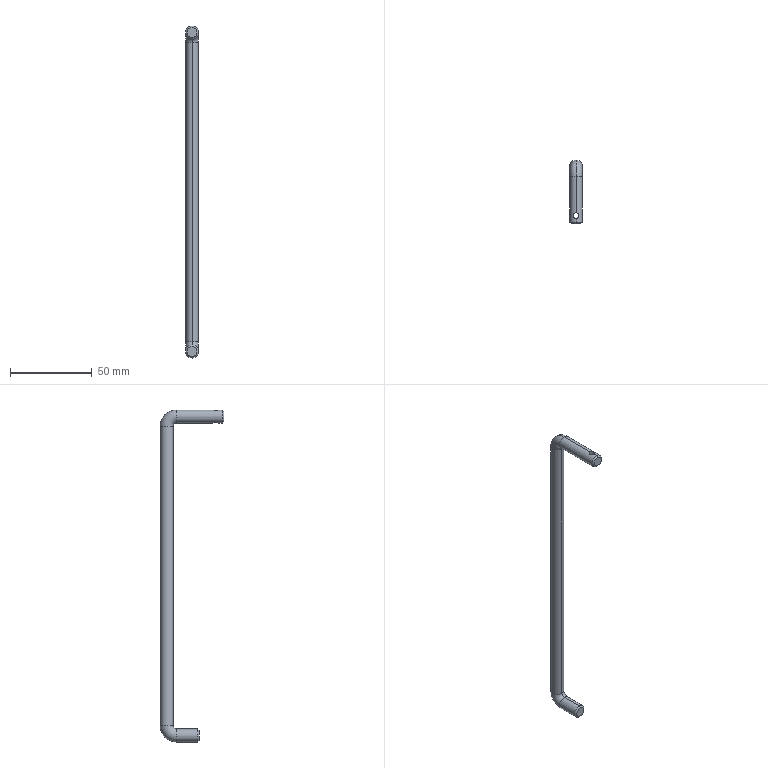Part | SolidWorks | features BaseBody 1 | 1 solid | 18 faces | box 8 x 39 x 203 mm | volume 12209 mm3 | cylinder 8 | cone 4 | torus 4 | plane 2 | commonest cylinder face diameters 8 x6 3.5 x2
STEP:
#1=CARTESIAN_POINT('',(1.75,-30.,101.097));
#2=VERTEX_POINT('',#1);
#3=CARTESIAN_POINT('',(1.75,-30.,93.903));
#4=VERTEX_POINT('',#3);
#5=CARTESIAN_POINT('',(1.75,-30.,132.));
#6=DIRECTION('',(0.,0.,-1.));
#7=VECTOR('',#6,1000.);
#8=LINE('',#5,#7);
#9=EDGE_CURVE('',#2,#4,#8,.T.);
#10=ORIENTED_EDGE('',*,*,#9,.F.);
#11=CARTESIAN_POINT('',(0.,-28.25,101.5));
#12=VERTEX_POINT('',#11);
#13=CARTESIAN_POINT('',(0.,-28.25,101.5));
#14=CARTESIAN_POINT('',(0.1167,-28.25,101.5));
#15=CARTESIAN_POINT('',(0.2317,-28.261,101.495));
#16=CARTESIAN_POINT('',(0.4573,-28.307,101.475));
#17=CARTESIAN_POINT('',(0.5697,-28.341,101.461));
#18=CARTESIAN_POINT('',(0.8889,-28.475,101.406));
#19=CARTESIAN_POINT('',(1.075,-28.6,101.357));
#20=CARTESIAN_POINT('',(1.321,-28.847,101.276));
#21=CARTESIAN_POINT('',(1.393,-28.935,101.25));
#22=CARTESIAN_POINT('',(1.487,-29.075,101.213));
#23=CARTESIAN_POINT('',(1.516,-29.124,101.202));
#24=CARTESIAN_POINT('',(1.569,-29.223,101.179));
#25=CARTESIAN_POINT('',(1.593,-29.272,101.169));
#26=CARTESIAN_POINT('',(1.706,-29.544,101.119));
#27=CARTESIAN_POINT('',(1.75,-29.768,101.097));
#28=CARTESIAN_POINT('',(1.75,-30.,101.097));
#29=B_SPLINE_CURVE_WITH_KNOTS('',3,(#13,#14,#15,#16,#17,#18,#19,#20,#21,#22,#23,#24,#25,#26,#27,#28),.UNSPECIFIED.,.F.,.F.,(4,2,2,2,2,2,2,4),(0.,0.125,0.25,0.5,0.625,0.6875,0.75,1.),.UNSPECIFIED.);
#30=EDGE_CURVE('',#12,#2,#29,.T.);
#31=ORIENTED_EDGE('',*,*,#30,.F.);
#32=CARTESIAN_POINT('',(-1.75,-30.,101.097));
#33=VERTEX_POINT('',#32);
#34=CARTESIAN_POINT('',(-1.75,-30.,101.097));
#35=CARTESIAN_POINT('',(-1.75,-29.884,101.097));
#36=CARTESIAN_POINT('',(-1.739,-29.769,101.102));
#37=CARTESIAN_POINT('',(-1.705,-29.6,101.118));
#38=CARTESIAN_POINT('',(-1.691,-29.545,101.125));
#39=CARTESIAN_POINT('',(-1.666,-29.462,101.137));
#40=CARTESIAN_POINT('',(-1.656,-29.434,101.141));
#41=CARTESIAN_POINT('',(-1.636,-29.379,101.15));
#42=CARTESIAN_POINT('',(-1.625,-29.351,101.155));
#43=CARTESIAN_POINT('',(-1.571,-29.22,101.179));
#44=CARTESIAN_POINT('',(-1.516,-29.118,101.202));
#45=CARTESIAN_POINT('',(-1.389,-28.93,101.252));
#46=CARTESIAN_POINT('',(-1.317,-28.842,101.278));
#47=CARTESIAN_POINT('',(-1.157,-28.683,101.33));
#48=CARTESIAN_POINT('',(-1.07,-28.611,101.355));
#49=CARTESIAN_POINT('',(-0.9274,-28.515,101.391));
#50=CARTESIAN_POINT('',(-0.8785,-28.486,101.403));
#51=CARTESIAN_POINT('',(-0.7783,-28.432,101.424));
#52=CARTESIAN_POINT('',(-0.7286,-28.408,101.433));
#53=CARTESIAN_POINT('',(-0.4588,-28.295,101.48));
#54=CARTESIAN_POINT('',(-0.233,-28.25,101.5));
#55=CARTESIAN_POINT('',(0.,-28.25,101.5));
#56=B_SPLINE_CURVE_WITH_KNOTS('',3,(#34,#35,#36,#37,#38,#39,#40,#41,#42,#43,#44,#45,#46,#47,#48,#49,#50,#51,#52,#53,#54,#55),.UNSPECIFIED.,.F.,.F.,(4,2,2,2,2,2,2,2,2,2,4),(0.,0.125,0.1875,0.2187,0.25,0.375,0.5,0.625,0.6875,0.75,1.),.UNSPECIFIED.);
#57=EDGE_CURVE('',#33,#12,#56,.T.);
#58=ORIENTED_EDGE('',*,*,#57,.F.);
#59=CARTESIAN_POINT('',(-1.75,-30.,93.903));
#60=VERTEX_POINT('',#59);
#61=CARTESIAN_POINT('',(-1.75,-30.,132.));
#62=DIRECTION('',(0.,0.,-1.));
#63=VECTOR('',#62,1000.);
#64=LINE('',#61,#63);
#65=EDGE_CURVE('',#33,#60,#64,.T.);
#66=ORIENTED_EDGE('',*,*,#65,.T.);
#67=CARTESIAN_POINT('',(0.,-28.25,93.5));
#68=VERTEX_POINT('',#67);
#69=CARTESIAN_POINT('',(0.,-28.25,93.5));
#70=CARTESIAN_POINT('',(-0.1167,-28.25,93.5));
#71=CARTESIAN_POINT('',(-0.2317,-28.261,93.505));
#72=CARTESIAN_POINT('',(-0.4008,-28.295,93.52));
#73=CARTESIAN_POINT('',(-0.4567,-28.309,93.526));
#74=CARTESIAN_POINT('',(-0.5672,-28.343,93.54));
#75=CARTESIAN_POINT('',(-0.6233,-28.364,93.549));
#76=CARTESIAN_POINT('',(-0.7812,-28.43,93.576));
#77=CARTESIAN_POINT('',(-0.8823,-28.485,93.597));
#78=CARTESIAN_POINT('',(-1.072,-28.612,93.645));
#79=CARTESIAN_POINT('',(-1.159,-28.684,93.671));
#80=CARTESIAN_POINT('',(-1.319,-28.844,93.723));
#81=CARTESIAN_POINT('',(-1.39,-28.93,93.748));
#82=CARTESIAN_POINT('',(-1.486,-29.074,93.786));
#83=CARTESIAN_POINT('',(-1.515,-29.123,93.798));
#84=CARTESIAN_POINT('',(-1.556,-29.198,93.815));
#85=CARTESIAN_POINT('',(-1.568,-29.223,93.82));
#86=CARTESIAN_POINT('',(-1.593,-29.274,93.831));
#87=CARTESIAN_POINT('',(-1.604,-29.299,93.836));
#88=CARTESIAN_POINT('',(-1.706,-29.543,93.881));
#89=CARTESIAN_POINT('',(-1.75,-29.768,93.903));
#90=CARTESIAN_POINT('',(-1.75,-30.,93.903));
#91=B_SPLINE_CURVE_WITH_KNOTS('',3,(#69,#70,#71,#72,#73,#74,#75,#76,#77,#78,#79,#80,#81,#82,#83,#84,#85,#86,#87,#88,#89,#90),.UNSPECIFIED.,.F.,.F.,(4,2,2,2,2,2,2,2,2,2,4),(0.,0.125,0.1875,0.25,0.375,0.5,0.625,0.6875,0.7187,0.75,1.),.UNSPECIFIED.);
#92=EDGE_CURVE('',#68,#60,#91,.T.);
#93=ORIENTED_EDGE('',*,*,#92,.F.);
#94=CARTESIAN_POINT('',(1.75,-30.,93.903));
#95=CARTESIAN_POINT('',(1.75,-29.77,93.903));
#96=CARTESIAN_POINT('',(1.703,-29.536,93.879));
#97=CARTESIAN_POINT('',(1.571,-29.221,93.821));
#98=CARTESIAN_POINT('',(1.518,-29.121,93.799));
#99=CARTESIAN_POINT('',(1.393,-28.934,93.75));
#100=CARTESIAN_POINT('',(1.319,-28.844,93.723));
#101=CARTESIAN_POINT('',(1.157,-28.682,93.67));
#102=CARTESIAN_POINT('',(1.069,-28.61,93.644));
#103=CARTESIAN_POINT('',(0.8816,-28.484,93.597));
#104=CARTESIAN_POINT('',(0.7831,-28.431,93.576));
#105=CARTESIAN_POINT('',(0.4592,-28.295,93.52));
#106=CARTESIAN_POINT('',(0.2331,-28.25,93.5));
#107=CARTESIAN_POINT('',(0.,-28.25,93.5));
#108=B_SPLINE_CURVE_WITH_KNOTS('',3,(#94,#95,#96,#97,#98,#99,#100,#101,#102,#103,#104,#105,#106,#107),.UNSPECIFIED.,.F.,.F.,(4,2,2,2,2,2,4),(0.,0.25,0.375,0.5,0.625,0.75,1.),.UNSPECIFIED.);
#109=EDGE_CURVE('',#4,#68,#108,.T.);
#110=ORIENTED_EDGE('',*,*,#109,.F.);
#111=EDGE_LOOP('',(#10,#31,#58,#66,#93,#110));
#112=FACE_OUTER_BOUND('',#111,.T.);
#113=CARTESIAN_POINT('',(0.,-30.,132.));
#114=DIRECTION('',(0.,0.,-1.));
#115=DIRECTION('',(-1.,0.,0.));
#116=AXIS2_PLACEMENT_3D('',#113,#114,#115);
#117=CYLINDRICAL_SURFACE('',#116,1.75);
#118=ADVANCED_FACE('',(#112),#117,.F.);
#119=CARTESIAN_POINT('',(0.,-35.,94.5));
#120=VERTEX_POINT('',#119);
#121=CARTESIAN_POINT('',(0.,-34.,93.5));
#122=VERTEX_POINT('',#121);
#123=CARTESIAN_POINT('',(0.,-35.,94.5));
#124=DIRECTION('',(0.,0.7071,-0.7071));
#125=VECTOR('',#124,1000.);
#126=LINE('',#123,#125);
#127=EDGE_CURVE('',#120,#122,#126,.T.);
#128=ORIENTED_EDGE('',*,*,#127,.F.);
#129=CARTESIAN_POINT('',(0.,-35.,100.5));
#130=VERTEX_POINT('',#129);
#131=CARTESIAN_POINT('',(0.,-35.,97.5));
#132=DIRECTION('',(0.,-1.,0.));
#133=DIRECTION('',(0.,0.,-1.));
#134=AXIS2_PLACEMENT_3D('',#131,#132,#133);
#135=CIRCLE('',#134,3.);
#136=EDGE_CURVE('',#130,#120,#135,.T.);
#137=ORIENTED_EDGE('',*,*,#136,.F.);
#138=CARTESIAN_POINT('',(0.,-34.,101.5));
#139=VERTEX_POINT('',#138);
#140=CARTESIAN_POINT('',(0.,-35.,100.5));
#141=DIRECTION('',(0.,0.7071,0.7071));
#142=VECTOR('',#141,1000.);
#143=LINE('',#140,#142);
#144=EDGE_CURVE('',#130,#139,#143,.T.);
#145=ORIENTED_EDGE('',*,*,#144,.T.);
#146=CARTESIAN_POINT('',(0.,-34.,97.5));
#147=DIRECTION('',(0.,1.,0.));
#148=DIRECTION('',(0.,0.,-1.));
#149=AXIS2_PLACEMENT_3D('',#146,#147,#148);
#150=CIRCLE('',#149,4.);
#151=EDGE_CURVE('',#122,#139,#150,.T.);
#152=ORIENTED_EDGE('',*,*,#151,.F.);
#153=EDGE_LOOP('',(#128,#137,#145,#152));
#154=FACE_OUTER_BOUND('',#153,.T.);
#155=CARTESIAN_POINT('',(0.,-35.,97.5));
#156=DIRECTION('',(0.,1.,0.));
#157=DIRECTION('',(0.,0.,1.));
#158=AXIS2_PLACEMENT_3D('',#155,#156,#157);
#159=CONICAL_SURFACE('',#158,3.,0.7854);
#160=ADVANCED_FACE('',(#154),#159,.T.);
#161=CARTESIAN_POINT('',(0.,-20.,-100.5));
#162=VERTEX_POINT('',#161);
#163=CARTESIAN_POINT('',(0.,-19.,-101.5));
#164=VERTEX_POINT('',#163);
#165=CARTESIAN_POINT('',(0.,-19.,-101.5));
#166=DIRECTION('',(0.,0.7071,-0.7071));
#167=VECTOR('',#166,1000.);
#168=LINE('',#165,#167);
#169=EDGE_CURVE('',#162,#164,#168,.T.);
#170=ORIENTED_EDGE('',*,*,#169,.F.);
#171=CARTESIAN_POINT('',(0.,-20.,-94.5));
#172=VERTEX_POINT('',#171);
#173=CARTESIAN_POINT('',(0.,-20.,-97.5));
#174=DIRECTION('',(0.,-1.,0.));
#175=DIRECTION('',(0.,0.,1.));
#176=AXIS2_PLACEMENT_3D('',#173,#174,#175);
#177=CIRCLE('',#176,3.);
#178=EDGE_CURVE('',#172,#162,#177,.T.);
#179=ORIENTED_EDGE('',*,*,#178,.F.);
#180=CARTESIAN_POINT('',(0.,-19.,-93.5));
#181=VERTEX_POINT('',#180);
#182=CARTESIAN_POINT('',(0.,-19.,-93.5));
#183=DIRECTION('',(0.,0.7071,0.7071));
#184=VECTOR('',#183,1000.);
#185=LINE('',#182,#184);
#186=EDGE_CURVE('',#172,#181,#185,.T.);
#187=ORIENTED_EDGE('',*,*,#186,.T.);
#188=CARTESIAN_POINT('',(0.,-19.,-97.5));
#189=DIRECTION('',(0.,1.,0.));
#190=DIRECTION('',(0.,0.,1.));
#191=AXIS2_PLACEMENT_3D('',#188,#189,#190);
#192=CIRCLE('',#191,4.);
#193=EDGE_CURVE('',#164,#181,#192,.T.);
#194=ORIENTED_EDGE('',*,*,#193,.F.);
#195=EDGE_LOOP('',(#170,#179,#187,#194));
#196=FACE_OUTER_BOUND('',#195,.T.);
#197=CARTESIAN_POINT('',(0.,-19.,-97.5));
#198=DIRECTION('',(0.,1.,0.));
#199=DIRECTION('',(0.,0.,1.));
#200=AXIS2_PLACEMENT_3D('',#197,#198,#199);
#201=CONICAL_SURFACE('',#200,4.,0.7854);
#202=ADVANCED_FACE('',(#196),#201,.T.);
#203=ORIENTED_EDGE('',*,*,#178,.T.);
#204=CARTESIAN_POINT('',(0.,-20.,-97.5));
#205=DIRECTION('',(0.,-1.,0.));
#206=DIRECTION('',(0.,0.,1.));
#207=AXIS2_PLACEMENT_3D('',#204,#205,#206);
#208=CIRCLE('',#207,3.);
#209=EDGE_CURVE('',#162,#172,#208,.T.);
#210=ORIENTED_EDGE('',*,*,#209,.T.);
#211=EDGE_LOOP('',(#203,#210));
#212=FACE_OUTER_BOUND('',#211,.T.);
#213=CARTESIAN_POINT('',(0.,-20.,-97.5));
#214=DIRECTION('',(0.,1.,0.));
#215=DIRECTION('',(0.,0.,-1.));
#216=AXIS2_PLACEMENT_3D('',#213,#214,#215);
#217=PLANE('',#216);
#218=ADVANCED_FACE('',(#212),#217,.F.);
#219=ORIENTED_EDGE('',*,*,#136,.T.);
#220=CARTESIAN_POINT('',(0.,-35.,97.5));
#221=DIRECTION('',(0.,-1.,0.));
#222=DIRECTION('',(0.,0.,-1.));
#223=AXIS2_PLACEMENT_3D('',#220,#221,#222);
#224=CIRCLE('',#223,3.);
#225=EDGE_CURVE('',#120,#130,#224,.T.);
#226=ORIENTED_EDGE('',*,*,#225,.T.);
#227=EDGE_LOOP('',(#219,#226));
#228=FACE_OUTER_BOUND('',#227,.T.);
#229=CARTESIAN_POINT('',(0.,-35.,97.5));
#230=DIRECTION('',(0.,-1.,0.));
#231=DIRECTION('',(0.,0.,-1.));
#232=AXIS2_PLACEMENT_3D('',#229,#230,#231);
#233=PLANE('',#232);
#234=ADVANCED_FACE('',(#228),#233,.T.);
#235=CARTESIAN_POINT('',(0.,-6.,-101.5));
#236=VERTEX_POINT('',#235);
#237=CARTESIAN_POINT('',(0.,-20.,-101.5));
#238=DIRECTION('',(0.,1.,0.));
#239=VECTOR('',#238,1000.);
#240=LINE('',#237,#239);
#241=EDGE_CURVE('',#164,#236,#240,.T.);
#242=ORIENTED_EDGE('',*,*,#241,.F.);
#243=ORIENTED_EDGE('',*,*,#193,.T.);
#244=CARTESIAN_POINT('',(0.,-6.,-93.5));
#245=VERTEX_POINT('',#244);
#246=CARTESIAN_POINT('',(0.,-20.,-93.5));
#247=DIRECTION('',(0.,1.,0.));
#248=VECTOR('',#247,1000.);
#249=LINE('',#246,#248);
#250=EDGE_CURVE('',#181,#245,#249,.T.);
#251=ORIENTED_EDGE('',*,*,#250,.T.);
#252=CARTESIAN_POINT('',(0.,-6.,-97.5));
#253=DIRECTION('',(0.,1.,0.));
#254=DIRECTION('',(1.,0.,0.));
#255=AXIS2_PLACEMENT_3D('',#252,#253,#254);
#256=CIRCLE('',#255,4.);
#257=EDGE_CURVE('',#236,#245,#256,.T.);
#258=ORIENTED_EDGE('',*,*,#257,.F.);
#259=EDGE_LOOP('',(#242,#243,#251,#258));
#260=FACE_OUTER_BOUND('',#259,.T.);
#261=CARTESIAN_POINT('',(0.,-20.,-97.5));
#262=DIRECTION('',(0.,1.,0.));
#263=DIRECTION('',(0.,0.,1.));
#264=AXIS2_PLACEMENT_3D('',#261,#262,#263);
#265=CYLINDRICAL_SURFACE('',#264,4.);
#266=ADVANCED_FACE('',(#260),#265,.T.);
#267=CARTESIAN_POINT('',(0.,4.,-91.5));
#268=VERTEX_POINT('',#267);
#269=CARTESIAN_POINT('',(0.,-6.,-91.5));
#270=DIRECTION('',(1.,0.,0.));
#271=DIRECTION('',(0.,0.,-1.));
#272=AXIS2_PLACEMENT_3D('',#269,#270,#271);
#273=CIRCLE('',#272,10.);
#274=EDGE_CURVE('',#236,#268,#273,.T.);
#275=ORIENTED_EDGE('',*,*,#274,.F.);
#276=ORIENTED_EDGE('',*,*,#257,.T.);
#277=CARTESIAN_POINT('',(0.,-4.,-91.5));
#278=VERTEX_POINT('',#277);
#279=CARTESIAN_POINT('',(0.,-6.,-91.5));
#280=DIRECTION('',(1.,0.,0.));
#281=DIRECTION('',(0.,0.,-1.));
#282=AXIS2_PLACEMENT_3D('',#279,#280,#281);
#283=CIRCLE('',#282,2.);
#284=EDGE_CURVE('',#245,#278,#283,.T.);
#285=ORIENTED_EDGE('',*,*,#284,.T.);
#286=CARTESIAN_POINT('',(0.,0.,-91.5));
#287=DIRECTION('',(0.,0.,1.));
#288=DIRECTION('',(1.,0.,0.));
#289=AXIS2_PLACEMENT_3D('',#286,#287,#288);
#290=CIRCLE('',#289,4.);
#291=EDGE_CURVE('',#268,#278,#290,.T.);
#292=ORIENTED_EDGE('',*,*,#291,.F.);
#293=EDGE_LOOP('',(#275,#276,#285,#292));
#294=FACE_OUTER_BOUND('',#293,.T.);
#295=CARTESIAN_POINT('',(0.,-6.,-91.5));
#296=DIRECTION('',(1.,0.,0.));
#297=DIRECTION('',(0.,0.,-1.));
#298=AXIS2_PLACEMENT_3D('',#295,#296,#297);
#299=TOROIDAL_SURFACE('',#298,6.,4.);
#300=ADVANCED_FACE('',(#294),#299,.T.);
#301=CARTESIAN_POINT('',(0.,4.,91.5));
#302=VERTEX_POINT('',#301);
#303=CARTESIAN_POINT('',(0.,4.,-91.5));
#304=DIRECTION('',(0.,0.,1.));
#305=VECTOR('',#304,1000.);
#306=LINE('',#303,#305);
#307=EDGE_CURVE('',#268,#302,#306,.T.);
#308=ORIENTED_EDGE('',*,*,#307,.F.);
#309=ORIENTED_EDGE('',*,*,#291,.T.);
#310=CARTESIAN_POINT('',(0.,-4.,91.5));
#311=VERTEX_POINT('',#310);
#312=CARTESIAN_POINT('',(0.,-4.,-91.5));
#313=DIRECTION('',(0.,0.,1.));
#314=VECTOR('',#313,1000.);
#315=LINE('',#312,#314);
#316=EDGE_CURVE('',#278,#311,#315,.T.);
#317=ORIENTED_EDGE('',*,*,#316,.T.);
#318=CARTESIAN_POINT('',(0.,0.,91.5));
#319=DIRECTION('',(0.,0.,1.));
#320=DIRECTION('',(1.,0.,0.));
#321=AXIS2_PLACEMENT_3D('',#318,#319,#320);
#322=CIRCLE('',#321,4.);
#323=EDGE_CURVE('',#302,#311,#322,.T.);
#324=ORIENTED_EDGE('',*,*,#323,.F.);
#325=EDGE_LOOP('',(#308,#309,#317,#324));
#326=FACE_OUTER_BOUND('',#325,.T.);
#327=CARTESIAN_POINT('',(0.,0.,-91.5));
#328=DIRECTION('',(0.,0.,1.));
#329=DIRECTION('',(0.,-1.,0.));
#330=AXIS2_PLACEMENT_3D('',#327,#328,#329);
#331=CYLINDRICAL_SURFACE('',#330,4.);
#332=ADVANCED_FACE('',(#326),#331,.T.);
#333=CARTESIAN_POINT('',(0.,-6.,101.5));
#334=VERTEX_POINT('',#333);
#335=CARTESIAN_POINT('',(0.,-6.,91.5));
#336=DIRECTION('',(1.,0.,0.));
#337=DIRECTION('',(0.,0.,-1.));
#338=AXIS2_PLACEMENT_3D('',#335,#336,#337);
#339=CIRCLE('',#338,10.);
#340=EDGE_CURVE('',#302,#334,#339,.T.);
#341=ORIENTED_EDGE('',*,*,#340,.F.);
#342=ORIENTED_EDGE('',*,*,#323,.T.);
#343=CARTESIAN_POINT('',(0.,-6.,93.5));
#344=VERTEX_POINT('',#343);
#345=CARTESIAN_POINT('',(0.,-6.,91.5));
#346=DIRECTION('',(1.,0.,0.));
#347=DIRECTION('',(0.,0.,-1.));
#348=AXIS2_PLACEMENT_3D('',#345,#346,#347);
#349=CIRCLE('',#348,2.);
#350=EDGE_CURVE('',#311,#344,#349,.T.);
#351=ORIENTED_EDGE('',*,*,#350,.T.);
#352=CARTESIAN_POINT('',(0.,-6.,97.5));
#353=DIRECTION('',(0.,-1.,0.));
#354=DIRECTION('',(1.,0.,0.));
#355=AXIS2_PLACEMENT_3D('',#352,#353,#354);
#356=CIRCLE('',#355,4.);
#357=EDGE_CURVE('',#334,#344,#356,.T.);
#358=ORIENTED_EDGE('',*,*,#357,.F.);
#359=EDGE_LOOP('',(#341,#342,#351,#358));
#360=FACE_OUTER_BOUND('',#359,.T.);
#361=CARTESIAN_POINT('',(0.,-6.,91.5));
#362=DIRECTION('',(1.,0.,0.));
#363=DIRECTION('',(0.,0.,-1.));
#364=AXIS2_PLACEMENT_3D('',#361,#362,#363);
#365=TOROIDAL_SURFACE('',#364,6.,4.);
#366=ADVANCED_FACE('',(#360),#365,.T.);
#367=CARTESIAN_POINT('',(0.,-6.,101.5));
#368=DIRECTION('',(0.,-1.,0.));
#369=VECTOR('',#368,1000.);
#370=LINE('',#367,#369);
#371=EDGE_CURVE('',#334,#12,#370,.T.);
#372=ORIENTED_EDGE('',*,*,#371,.F.);
#373=ORIENTED_EDGE('',*,*,#357,.T.);
#374=CARTESIAN_POINT('',(0.,-6.,93.5));
#375=DIRECTION('',(0.,-1.,0.));
#376=VECTOR('',#375,1000.);
#377=LINE('',#374,#376);
#378=EDGE_CURVE('',#344,#68,#377,.T.);
#379=ORIENTED_EDGE('',*,*,#378,.T.);
#380=ORIENTED_EDGE('',*,*,#92,.T.);
#381=CARTESIAN_POINT('',(0.,-31.75,93.5));
#382=VERTEX_POINT('',#381);
#383=CARTESIAN_POINT('',(-1.75,-30.,93.903));
#384=CARTESIAN_POINT('',(-1.75,-30.116,93.903));
#385=CARTESIAN_POINT('',(-1.739,-30.231,93.898));
#386=CARTESIAN_POINT('',(-1.705,-30.4,93.882));
#387=CARTESIAN_POINT('',(-1.691,-30.455,93.875));
#388=CARTESIAN_POINT('',(-1.657,-30.566,93.859));
#389=CARTESIAN_POINT('',(-1.636,-30.623,93.85));
#390=CARTESIAN_POINT('',(-1.57,-30.781,93.821));
#391=CARTESIAN_POINT('',(-1.517,-30.88,93.798));
#392=CARTESIAN_POINT('',(-1.392,-31.068,93.749));
#393=CARTESIAN_POINT('',(-1.318,-31.157,93.722));
#394=CARTESIAN_POINT('',(-1.155,-31.319,93.67));
#395=CARTESIAN_POINT('',(-1.068,-31.391,93.644));
#396=CARTESIAN_POINT('',(-0.8804,-31.517,93.597));
#397=CARTESIAN_POINT('',(-0.7819,-31.57,93.576));
#398=CARTESIAN_POINT('',(-0.4584,-31.705,93.52));
#399=CARTESIAN_POINT('',(-0.2328,-31.75,93.5));
#400=CARTESIAN_POINT('',(0.,-31.75,93.5));
#401=B_SPLINE_CURVE_WITH_KNOTS('',3,(#383,#384,#385,#386,#387,#388,#389,#390,#391,#392,#393,#394,#395,#396,#397,#398,#399,#400),.UNSPECIFIED.,.F.,.F.,(4,2,2,2,2,2,2,2,4),(0.,0.125,0.1875,0.25,0.375,0.5,0.625,0.75,1.),.UNSPECIFIED.);
#402=EDGE_CURVE('',#60,#382,#401,.T.);
#403=ORIENTED_EDGE('',*,*,#402,.T.);
#404=CARTESIAN_POINT('',(0.,-6.,93.5));
#405=DIRECTION('',(0.,-1.,0.));
#406=VECTOR('',#405,1000.);
#407=LINE('',#404,#406);
#408=EDGE_CURVE('',#382,#122,#407,.T.);
#409=ORIENTED_EDGE('',*,*,#408,.T.);
#410=ORIENTED_EDGE('',*,*,#151,.T.);
#411=CARTESIAN_POINT('',(0.,-31.75,101.5));
#412=VERTEX_POINT('',#411);
#413=CARTESIAN_POINT('',(0.,-6.,101.5));
#414=DIRECTION('',(0.,-1.,0.));
#415=VECTOR('',#414,1000.);
#416=LINE('',#413,#415);
#417=EDGE_CURVE('',#412,#139,#416,.T.);
#418=ORIENTED_EDGE('',*,*,#417,.F.);
#419=CARTESIAN_POINT('',(0.,-31.75,101.5));
#420=CARTESIAN_POINT('',(-0.1165,-31.75,101.5));
#421=CARTESIAN_POINT('',(-0.2312,-31.739,101.495));
#422=CARTESIAN_POINT('',(-0.4563,-31.694,101.475));
#423=CARTESIAN_POINT('',(-0.5683,-31.659,101.461));
#424=CARTESIAN_POINT('',(-0.7811,-31.57,101.424));
#425=CARTESIAN_POINT('',(-0.8813,-31.517,101.403));
#426=CARTESIAN_POINT('',(-1.069,-31.391,101.356));
#427=CARTESIAN_POINT('',(-1.156,-31.319,101.33));
#428=CARTESIAN_POINT('',(-1.32,-31.155,101.277));
#429=CARTESIAN_POINT('',(-1.393,-31.066,101.25));
#430=CARTESIAN_POINT('',(-1.486,-30.926,101.214));
#431=CARTESIAN_POINT('',(-1.515,-30.878,101.202));
#432=CARTESIAN_POINT('',(-1.569,-30.778,101.18));
#433=CARTESIAN_POINT('',(-1.592,-30.729,101.17));
#434=CARTESIAN_POINT('',(-1.706,-30.457,101.119));
#435=CARTESIAN_POINT('',(-1.75,-30.232,101.097));
#436=CARTESIAN_POINT('',(-1.75,-30.,101.097));
#437=B_SPLINE_CURVE_WITH_KNOTS('',3,(#419,#420,#421,#422,#423,#424,#425,#426,#427,#428,#429,#430,#431,#432,#433,#434,#435,#436),.UNSPECIFIED.,.F.,.F.,(4,2,2,2,2,2,2,2,4),(0.,0.125,0.25,0.375,0.5,0.625,0.6875,0.75,1.),.UNSPECIFIED.);
#438=EDGE_CURVE('',#412,#33,#437,.T.);
#439=ORIENTED_EDGE('',*,*,#438,.T.);
#440=ORIENTED_EDGE('',*,*,#57,.T.);
#441=EDGE_LOOP('',(#372,#373,#379,#380,#403,#409,#410,#418,#439,#440));
#442=FACE_OUTER_BOUND('',#441,.T.);
#443=CARTESIAN_POINT('',(0.,-6.,97.5));
#444=DIRECTION('',(0.,-1.,0.));
#445=DIRECTION('',(0.,0.,-1.));
#446=AXIS2_PLACEMENT_3D('',#443,#444,#445);
#447=CYLINDRICAL_SURFACE('',#446,4.);
#448=ADVANCED_FACE('',(#442),#447,.T.);
#449=CARTESIAN_POINT('',(0.,-6.,97.5));
#450=DIRECTION('',(0.,-1.,0.));
#451=DIRECTION('',(1.,0.,0.));
#452=AXIS2_PLACEMENT_3D('',#449,#450,#451);
#453=CIRCLE('',#452,4.);
#454=EDGE_CURVE('',#344,#334,#453,.T.);
#455=ORIENTED_EDGE('',*,*,#454,.T.);
#456=ORIENTED_EDGE('',*,*,#371,.T.);
#457=ORIENTED_EDGE('',*,*,#30,.T.);
#458=CARTESIAN_POINT('',(1.75,-30.,101.097));
#459=CARTESIAN_POINT('',(1.75,-30.116,101.097));
#460=CARTESIAN_POINT('',(1.739,-30.23,101.102));
#461=CARTESIAN_POINT('',(1.705,-30.399,101.118));
#462=CARTESIAN_POINT('',(1.691,-30.455,101.125));
#463=CARTESIAN_POINT('',(1.657,-30.565,101.141));
#464=CARTESIAN_POINT('',(1.637,-30.622,101.15));
#465=CARTESIAN_POINT('',(1.571,-30.78,101.179));
#466=CARTESIAN_POINT('',(1.518,-30.88,101.202));
#467=CARTESIAN_POINT('',(1.392,-31.067,101.251));
#468=CARTESIAN_POINT('',(1.318,-31.157,101.277));
#469=CARTESIAN_POINT('',(1.156,-31.319,101.33));
#470=CARTESIAN_POINT('',(1.068,-31.391,101.356));
#471=CARTESIAN_POINT('',(0.8805,-31.517,101.403));
#472=CARTESIAN_POINT('',(0.782,-31.57,101.424));
#473=CARTESIAN_POINT('',(0.4585,-31.705,101.48));
#474=CARTESIAN_POINT('',(0.2328,-31.75,101.5));
#475=CARTESIAN_POINT('',(0.,-31.75,101.5));
#476=B_SPLINE_CURVE_WITH_KNOTS('',3,(#458,#459,#460,#461,#462,#463,#464,#465,#466,#467,#468,#469,#470,#471,#472,#473,#474,#475),.UNSPECIFIED.,.F.,.F.,(4,2,2,2,2,2,2,2,4),(0.,0.125,0.1875,0.25,0.375,0.5,0.625,0.75,1.),.UNSPECIFIED.);
#477=EDGE_CURVE('',#2,#412,#476,.T.);
#478=ORIENTED_EDGE('',*,*,#477,.T.);
#479=ORIENTED_EDGE('',*,*,#417,.T.);
#480=CARTESIAN_POINT('',(0.,-34.,97.5));
#481=DIRECTION('',(0.,1.,0.));
#482=DIRECTION('',(0.,0.,-1.));
#483=AXIS2_PLACEMENT_3D('',#480,#481,#482);
#484=CIRCLE('',#483,4.);
#485=EDGE_CURVE('',#139,#122,#484,.T.);
#486=ORIENTED_EDGE('',*,*,#485,.T.);
#487=ORIENTED_EDGE('',*,*,#408,.F.);
#488=CARTESIAN_POINT('',(0.,-31.75,93.5));
#489=CARTESIAN_POINT('',(0.1166,-31.75,93.5));
#490=CARTESIAN_POINT('',(0.2314,-31.739,93.505));
#491=CARTESIAN_POINT('',(0.4567,-31.694,93.525));
#492=CARTESIAN_POINT('',(0.5687,-31.659,93.539));
#493=CARTESIAN_POINT('',(0.8883,-31.525,93.594));
#494=CARTESIAN_POINT('',(1.075,-31.401,93.643));
#495=CARTESIAN_POINT('',(1.321,-31.154,93.723));
#496=CARTESIAN_POINT('',(1.393,-31.066,93.75));
#497=CARTESIAN_POINT('',(1.487,-30.925,93.787));
#498=CARTESIAN_POINT('',(1.516,-30.877,93.798));
#499=CARTESIAN_POINT('',(1.569,-30.777,93.82));
#500=CARTESIAN_POINT('',(1.593,-30.728,93.831));
#501=CARTESIAN_POINT('',(1.706,-30.456,93.881));
#502=CARTESIAN_POINT('',(1.75,-30.232,93.903));
#503=CARTESIAN_POINT('',(1.75,-30.,93.903));
#504=B_SPLINE_CURVE_WITH_KNOTS('',3,(#488,#489,#490,#491,#492,#493,#494,#495,#496,#497,#498,#499,#500,#501,#502,#503),.UNSPECIFIED.,.F.,.F.,(4,2,2,2,2,2,2,4),(0.,0.125,0.25,0.5,0.625,0.6875,0.75,1.),.UNSPECIFIED.);
#505=EDGE_CURVE('',#382,#4,#504,.T.);
#506=ORIENTED_EDGE('',*,*,#505,.T.);
#507=ORIENTED_EDGE('',*,*,#109,.T.);
#508=ORIENTED_EDGE('',*,*,#378,.F.);
#509=EDGE_LOOP('',(#455,#456,#457,#478,#479,#486,#487,#506,#507,#508));
#510=FACE_OUTER_BOUND('',#509,.T.);
#511=CARTESIAN_POINT('',(0.,-6.,97.5));
#512=DIRECTION('',(0.,-1.,0.));
#513=DIRECTION('',(0.,0.,-1.));
#514=AXIS2_PLACEMENT_3D('',#511,#512,#513);
#515=CYLINDRICAL_SURFACE('',#514,4.);
#516=ADVANCED_FACE('',(#510),#515,.T.);
#517=CARTESIAN_POINT('',(0.,-19.,-97.5));
#518=DIRECTION('',(0.,1.,0.));
#519=DIRECTION('',(0.,0.,1.));
#520=AXIS2_PLACEMENT_3D('',#517,#518,#519);
#521=CIRCLE('',#520,4.);
#522=EDGE_CURVE('',#181,#164,#521,.T.);
#523=ORIENTED_EDGE('',*,*,#522,.T.);
#524=ORIENTED_EDGE('',*,*,#241,.T.);
#525=CARTESIAN_POINT('',(0.,-6.,-97.5));
#526=DIRECTION('',(0.,1.,0.));
#527=DIRECTION('',(1.,0.,0.));
#528=AXIS2_PLACEMENT_3D('',#525,#526,#527);
#529=CIRCLE('',#528,4.);
#530=EDGE_CURVE('',#245,#236,#529,.T.);
#531=ORIENTED_EDGE('',*,*,#530,.F.);
#532=ORIENTED_EDGE('',*,*,#250,.F.);
#533=EDGE_LOOP('',(#523,#524,#531,#532));
#534=FACE_OUTER_BOUND('',#533,.T.);
#535=CARTESIAN_POINT('',(0.,-20.,-97.5));
#536=DIRECTION('',(0.,1.,0.));
#537=DIRECTION('',(0.,0.,1.));
#538=AXIS2_PLACEMENT_3D('',#535,#536,#537);
#539=CYLINDRICAL_SURFACE('',#538,4.);
#540=ADVANCED_FACE('',(#534),#539,.T.);
#541=CARTESIAN_POINT('',(0.,0.,-91.5));
#542=DIRECTION('',(0.,0.,1.));
#543=DIRECTION('',(1.,0.,0.));
#544=AXIS2_PLACEMENT_3D('',#541,#542,#543);
#545=CIRCLE('',#544,4.);
#546=EDGE_CURVE('',#278,#268,#545,.T.);
#547=ORIENTED_EDGE('',*,*,#546,.T.);
#548=ORIENTED_EDGE('',*,*,#307,.T.);
#549=CARTESIAN_POINT('',(0.,0.,91.5));
#550=DIRECTION('',(0.,0.,1.));
#551=DIRECTION('',(1.,0.,0.));
#552=AXIS2_PLACEMENT_3D('',#549,#550,#551);
#553=CIRCLE('',#552,4.);
#554=EDGE_CURVE('',#311,#302,#553,.T.);
#555=ORIENTED_EDGE('',*,*,#554,.F.);
#556=ORIENTED_EDGE('',*,*,#316,.F.);
#557=EDGE_LOOP('',(#547,#548,#555,#556));
#558=FACE_OUTER_BOUND('',#557,.T.);
#559=CARTESIAN_POINT('',(0.,0.,-91.5));
#560=DIRECTION('',(0.,0.,1.));
#561=DIRECTION('',(0.,-1.,0.));
#562=AXIS2_PLACEMENT_3D('',#559,#560,#561);
#563=CYLINDRICAL_SURFACE('',#562,4.);
#564=ADVANCED_FACE('',(#558),#563,.T.);
#565=ORIENTED_EDGE('',*,*,#209,.F.);
#566=ORIENTED_EDGE('',*,*,#169,.T.);
#567=ORIENTED_EDGE('',*,*,#522,.F.);
#568=ORIENTED_EDGE('',*,*,#186,.F.);
#569=EDGE_LOOP('',(#565,#566,#567,#568));
#570=FACE_OUTER_BOUND('',#569,.T.);
#571=CARTESIAN_POINT('',(0.,-19.,-97.5));
#572=DIRECTION('',(0.,1.,0.));
#573=DIRECTION('',(0.,0.,1.));
#574=AXIS2_PLACEMENT_3D('',#571,#572,#573);
#575=CONICAL_SURFACE('',#574,4.,0.7854);
#576=ADVANCED_FACE('',(#570),#575,.T.);
#577=ORIENTED_EDGE('',*,*,#225,.F.);
#578=ORIENTED_EDGE('',*,*,#127,.T.);
#579=ORIENTED_EDGE('',*,*,#485,.F.);
#580=ORIENTED_EDGE('',*,*,#144,.F.);
#581=EDGE_LOOP('',(#577,#578,#579,#580));
#582=FACE_OUTER_BOUND('',#581,.T.);
#583=CARTESIAN_POINT('',(0.,-35.,97.5));
#584=DIRECTION('',(0.,1.,0.));
#585=DIRECTION('',(0.,0.,1.));
#586=AXIS2_PLACEMENT_3D('',#583,#584,#585);
#587=CONICAL_SURFACE('',#586,3.,0.7854);
#588=ADVANCED_FACE('',(#582),#587,.T.);
#589=ORIENTED_EDGE('',*,*,#477,.F.);
#590=ORIENTED_EDGE('',*,*,#9,.T.);
#591=ORIENTED_EDGE('',*,*,#505,.F.);
#592=ORIENTED_EDGE('',*,*,#402,.F.);
#593=ORIENTED_EDGE('',*,*,#65,.F.);
#594=ORIENTED_EDGE('',*,*,#438,.F.);
#595=EDGE_LOOP('',(#589,#590,#591,#592,#593,#594));
#596=FACE_OUTER_BOUND('',#595,.T.);
#597=CARTESIAN_POINT('',(0.,-30.,132.));
#598=DIRECTION('',(0.,0.,-1.));
#599=DIRECTION('',(-1.,0.,0.));
#600=AXIS2_PLACEMENT_3D('',#597,#598,#599);
#601=CYLINDRICAL_SURFACE('',#600,1.75);
#602=ADVANCED_FACE('',(#596),#601,.F.);
#603=ORIENTED_EDGE('',*,*,#530,.T.);
#604=ORIENTED_EDGE('',*,*,#274,.T.);
#605=ORIENTED_EDGE('',*,*,#546,.F.);
#606=ORIENTED_EDGE('',*,*,#284,.F.);
#607=EDGE_LOOP('',(#603,#604,#605,#606));
#608=FACE_OUTER_BOUND('',#607,.T.);
#609=CARTESIAN_POINT('',(0.,-6.,-91.5));
#610=DIRECTION('',(1.,0.,0.));
#611=DIRECTION('',(0.,0.,-1.));
#612=AXIS2_PLACEMENT_3D('',#609,#610,#611);
#613=TOROIDAL_SURFACE('',#612,6.,4.);
#614=ADVANCED_FACE('',(#608),#613,.T.);
#615=ORIENTED_EDGE('',*,*,#554,.T.);
#616=ORIENTED_EDGE('',*,*,#340,.T.);
#617=ORIENTED_EDGE('',*,*,#454,.F.);
#618=ORIENTED_EDGE('',*,*,#350,.F.);
#619=EDGE_LOOP('',(#615,#616,#617,#618));
#620=FACE_OUTER_BOUND('',#619,.T.);
#621=CARTESIAN_POINT('',(0.,-6.,91.5));
#622=DIRECTION('',(1.,0.,0.));
#623=DIRECTION('',(0.,0.,-1.));
#624=AXIS2_PLACEMENT_3D('',#621,#622,#623);
#625=TOROIDAL_SURFACE('',#624,6.,4.);
#626=ADVANCED_FACE('',(#620),#625,.T.);
#627=CLOSED_SHELL('',(#118,#160,#202,#218,#234,#266,#300,#332,#366,#448,#516,#540,#564,#576,#588,#602,#614,#626));
#628=MANIFOLD_SOLID_BREP('',#627);
#629=CARTESIAN_POINT('',(0.,0.,0.));
#630=DIRECTION('',(0.,0.,1.));
#631=DIRECTION('',(1.,0.,0.));
#632=AXIS2_PLACEMENT_3D('',#629,#630,#631);
#633=(LENGTH_UNIT()NAMED_UNIT(*)SI_UNIT(.MILLI.,.METRE.));
#634=UNCERTAINTY_MEASURE_WITH_UNIT(LENGTH_MEASURE(0.00001),#633,'','');
#635=(NAMED_UNIT(*)PLANE_ANGLE_UNIT()SI_UNIT($,.RADIAN.));
#636=(NAMED_UNIT(*)SI_UNIT($,.STERADIAN.)SOLID_ANGLE_UNIT());
#637=(GEOMETRIC_REPRESENTATION_CONTEXT(3)GLOBAL_UNCERTAINTY_ASSIGNED_CONTEXT((#634))GLOBAL_UNIT_ASSIGNED_CONTEXT((#633,#635,#636))REPRESENTATION_CONTEXT('',''));
#638=ADVANCED_BREP_SHAPE_REPRESENTATION('',(#628,#632),#637);